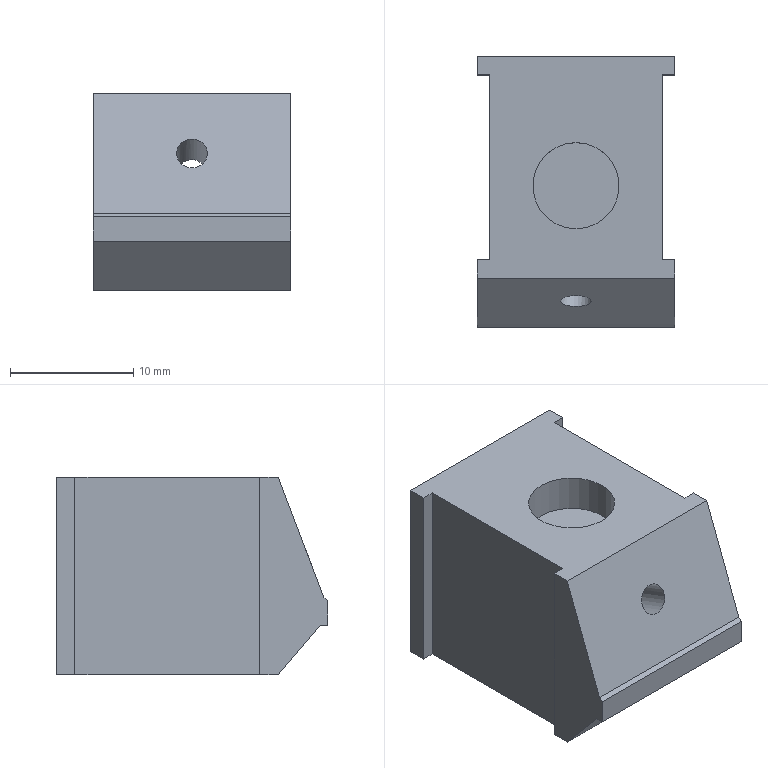Part | STEP file | 1-54.6 | 1 solid | 23 faces | box 16 x 22 x 16 mm | volume 3574 mm3 | plane 20 | cylinder 3 | commonest cylinder face diameters 2.5 x1 7 x1 9 x1